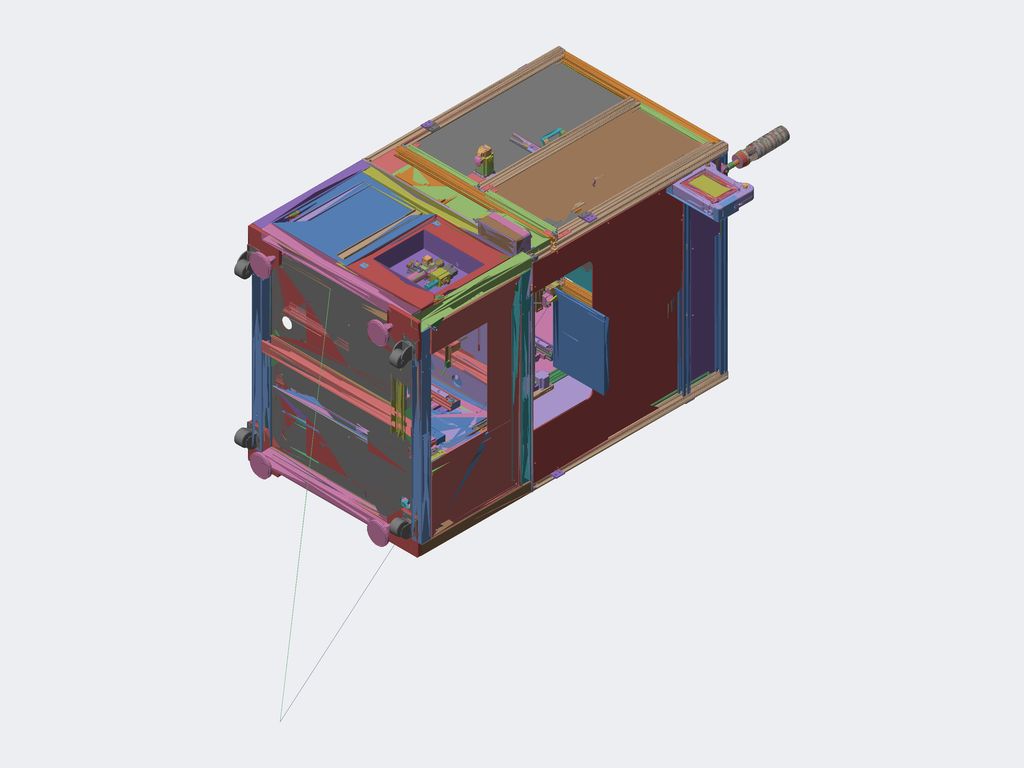Assembly | STEP file | 311 different items | 1352 placed
Parts list (item | name | quantity | parent item | size | volume):
1 | - | x3 | in standard line | 295.5 x 37 x 54 mm | 476987 mm3
2 | computer numeric keypad HW098A | x1 | - | 285 x 134.477 x 20.707 mm | 348145 mm3
3 | TOPNIKE 1205 aluminium handle, hole spacing 32mm | x1 | - | 7.369 x 16.8 x 50 mm | 4040 mm3
4 | NdFeB round magnet D12X3 with 3mm hole | x2 | - | 2.7 x 12 x 12 mm | 255.164 mm3
5 | aluminium profile door-catch magnet post | x4 | - | 14 x 14 x 37 mm | 3124 mm3
6 | monitor mounting plate | x1 | - | 92.213 x 406.803 x 260 mm | 560601 mm3
7 | magnet mounting plate | x1 | - | 20 x 12 x 35 mm | 1365 mm3
8 | smoke vent cover plate | x2 | - | 105 x 105 x 5 mm | 42706 mm3
9 | power strip mounting plate | x1 | - | 320 x 80 x 3 mm | 76368 mm3
10 | - | x4 | - | 45 x 17 x 40 mm | 3748 mm3
11 | organic panel mounting plate | x4 | - | 17 x 15 x 17 mm | 789.05 mm3
12 | - | x1 | - | 164 x 17 x 160 mm | 59024 mm3
13 | keyboard and mouse push plate | x1 | - | 14 x 138 x 548 mm | 182409 mm3
14 | 3030 L-profile sheet metal | x16 | - | 85 x 85 x 2.5 mm | 9017 mm3
15 | end cap panel MK-EC-B-4040x4.2 | x4 | in upper bracket frame assembly | 40 x 12.4 x 40 mm | 5038 mm3
16 | MK-8-4040C-L-01 profile 4040C standard 1145mm | x4 | in upper bracket frame assembly | 1145 x 40 x 40 mm | 545459 mm3
17 | - | x4 | in upper bracket frame assembly | 1120 x 40 x 40 mm | 531368 mm3
18 | MK-8-4040C-L-04 profile 4040C standard 920mm | x5 | in upper bracket frame assembly | 920 x 40 x 40 mm | 435718 mm3
19 | - | x4 | in rear door frame assembly | 1052 x 30 x 30 mm | 343124 mm3
20 | aluminium hinge 30_40 (incl. half-round hex socket bolt) | x8 | in rear door frame assembly, front door frame assembly | 66 x 54 x 16 mm | 29588 mm3
21 | - | x4 | in rear door frame assembly, front door frame assembly | 39 x 37 x 115 mm | 35258 mm3
22 | end cap panel MK-EC-B-3030x4 | x16 | in rear door frame assembly, front door frame assembly | 30 x 12.2 x 30 mm | 2778 mm3
23 | - | x8 | in rear door frame assembly, front door frame assembly | 397 x 30 x 30 mm | 129616 mm3
24 | M8x12 hex socket round-head bolt | x8 | in rear door frame assembly, front door frame assembly | 16.4 x 14 x 14 mm | 1090 mm3
25 | door panel | x2 | in rear door frame assembly | 1012 x 5 x 409 mm | 2069540 mm3
26 | MK-8-3030-L-99 profile 3030 standard 913mm | x4 | in front door frame assembly | 913 x 30 x 30 mm | 297727 mm3
27 | - | x3 | in upper bracket frame assembly | 20.75 x 39 x 18 mm | 5675 mm3
28 | - | x2 | - | 1119 x 884 x 5 mm | 3719703 mm3
29 | - | x2 | - | 1119 x 179 x 5 mm | 999682 mm3
30 | right front door acrylic cover plate | x1 | - | 870 x 409 x 5 mm | 1779111 mm3
31 | rear door acrylic cover plate | x2 | - | 1010 x 409 x 5 mm | 2065411 mm3
32 | left front door acrylic cover plate | x1 | - | 870 x 409 x 5 mm | 1779111 mm3
33 | - | x1 | - | 537 x 917 x 27.5 mm | 799133 mm3
34 | upper cover plate 2 | x1 | - | 537 x 917 x 27.5 mm | 772014 mm3
35 | spacer connection block MK-PMB-T-40 | x30 | - | 18 x 32 x 24 mm | 8600 mm3
36 | cable box hole plug φ60mm_light grey | x15 | in table top assembly | 70 x 70 x 12 mm | 8548 mm3
37 | - | x1 | - | 250 x 138 x 30 mm | 110009 mm3
38 | communication module connection plate | x1 | - | 120 x 138 x 30 mm | 59883 mm3
39 | - | x1 | - | - | -
40 | - | x1 | - | 290 x 245 x 56 mm | 381132 mm3
41 | - | x1 | - | 17.9 x 17.9 x 47.75 mm | 7538 mm3
42 | BZJ-LSX-TKJ 触摸屏MT8072iE_Default | x1 | - | - | -
43 | touch screen guide plate | x1 | - | 52 x 7.165 x 119.33 mm | 13457 mm3
44 | emergency stop button LAS1-AY-22TS-R | x1 | - | 23.995 x 49.1 x 23.995 mm | 9425 mm3
45 | - | x1 | - | 308.5 x 64.5 x 120 mm | 184454 mm3
46 | square proximity sensor GX-F12A | x4 | - | 12 x 47.7 x 8.8 mm | 2173 mm3
47 | - | x4 | - | 34.5 x 22.5 x 40 mm | 4337 mm3
48 | proximity switch mounting plate 2 | x4 | - | 40 x 32 x 18 mm | 3472 mm3
49 | display PANEL5000-IPM1502BT | x1 | - | - | -
50 | mouse | x1 | - | - | -
51 | - | x1 | - | 30.32 x 21 x 636 mm | 212983 mm3
52 | - | x2 | - | 11 x 5.5 x 5.5 mm | 119.075 mm3
53 | - | x16 | in lower bracket weldment 1000x1200 | 90 x 90 x 6 mm | 29274 mm3
54 | - | x4 | in lower bracket weldment 1000x1200 | 200 x 180 x 20 mm | 644827 mm3
55 | - | x1 | in lower bracket weldment 1000x1200 | 60 x 60 x 650 mm | 567586 mm3
56 | square steel tube 60x60x4x650 | x1 | in lower bracket weldment 1000x1200 | 60 x 60 x 650 mm | 567420 mm3
57 | square steel tube 60x60x4x880 | x2 | in lower bracket weldment 1000x1200 | 60 x 60 x 880 mm | 767950 mm3
58 | rear square steel tube 60x60x4x880 | x1 | in lower bracket weldment 1000x1200 | 60 x 60 x 880 mm | 769733 mm3
59 | - | x1 | in lower bracket weldment 1000x1200 | 60 x 60 x 880 mm | 769733 mm3
60 | - | x1 | in lower bracket weldment 1000x1200 | 60 x 60 x 1080 mm | 942814 mm3
61 | - | x1 | in lower bracket weldment 1000x1200 | 60 x 60 x 1080 mm | 943036 mm3
62 | square steel tube E60x60x4x1080 | x2 | in lower bracket weldment 1000x1200 | 60 x 60 x 1080 mm | 942050 mm3
63 | square steel tube F60x60x4x650 | x1 | in lower bracket weldment 1000x1200 | 60 x 60 x 650 mm | 567586 mm3
64 | square steel tube B60x60x4x880 | x2 | in lower bracket weldment 1000x1200 | 60 x 60 x 880 mm | 770145 mm3
65 | - | x1 | in lower bracket weldment 1000x1200 | 60 x 60 x 650 mm | 580718 mm3
66 | table plate | x1 | in lower bracket weldment 1000x1200 | 1000 x 1200 x 10 mm | 11534031 mm3
67 | - | x1 | in lower bracket weldment 1000x1200 | 45 x 5 x 105 mm | 23005 mm3
68 | spacer plate 4 | x1 | in lower bracket weldment 1000x1200 | 56 x 5 x 105 mm | 28583 mm3
69 | spacer plate 4 | x1 | in lower bracket weldment 1000x1200 | 56 x 5 x 105 mm | 28583 mm3
70 | - | x1 | in lower bracket weldment 1000x1200 | 45 x 5 x 105 mm | 23005 mm3
71 | - | x1 | in lower bracket weldment 1000x1200 | 105 x 5 x 105 mm | 53833 mm3
72 | - | x1 | in lower bracket weldment 1000x1200 | 105 x 5 x 105 mm | 53833 mm3
73 | - | x4 | in lower frame assembly 1000x1200 | 120 x 147 x 120 mm | 298172 mm3
74 | - | x4 | in lower frame assembly 1000x1200 | 112 x 105 x 88 mm | 158459 mm3
75 | - | x2 | in lower frame door assembly | 18 x 17 x 130 mm | 7934 mm3
76 | cylinder lock MS813-Shengjiu | x4 | in lower frame door assembly | 58.793 x 35 x 31.6 mm | 16415 mm3
77 | - | x2 | in lower frame door assembly | 15 x 20 x 350 mm | 20205 mm3
78 | - | x1 | - | 446.8 x 526 x 18.2 mm | 391845 mm3
79 | hinge CL237Z3H001-01 | x8 | in hinge CL237Z3H001 | 17.5 x 48 x 18 mm | 5234 mm3
80 | - | x8 | in hinge CL237Z3H001 | 19 x 25 x 8.5 mm | 1495 mm3
81 | - | x1 | - | 436 x 526 x 17 mm | 186343 mm3
82 | air source assembly mounting plate | x1 | - | 365 x 304.8 x 102 mm | 354021 mm3
83 | hand slide valve HSV08 | x1 | - | - | -
84 | - | x2 | - | 39.583 x 28.8 x 17.7 mm | 7284 mm3
85 | T-bracket GA300T-P1 | x1 | - | 60.5 x 88 x 12.5 mm | 30830 mm3
86 | soft-start valve GV30008JF1B | x1 | - | 57.4 x 130.9 x 74 mm | 252989 mm3
87 | plastic foam silencer PAL-03 | x1 | - | 26 x 68 x 26.213 mm | 26024 mm3
88 | pressure regulating filter GFR300-08-N | x1 | - | - | -
89 | digital pressure switch DP-102 | x1 | - | 30 x 30 x 44.8 mm | 24470 mm3
90 | countersunk screw spacer block | x16 | in lower frame bottom cover plate assembly, lower frame left cover plate assembly | 15 x 17 x 15 mm | 1639 mm3
91 | lower frame bottom cover plate | x2 | in lower frame bottom cover plate assembly | - | -
92 | lower frame left cover plate | x1 | in lower frame left cover plate assembly | 527 x 1077 x 15 mm | 446588 mm3
93 | - | x1 | - | 527 x 1077 x 15 mm | 446588 mm3
94 | table plate | x1 | in table top assembly | 1000 x 1200 x 10 mm | 11534031 mm3
95 | - | x10 | in assembled motion assembly | 15 x 18.7 x 22 mm | 803.602 mm3
96 | - | x5 | in assembled motion assembly | 15 x 19 x 15 mm | 469.105 mm3
97 | - | x5 | in assembled motion assembly | 35 x 35 x 10 mm | 7611 mm3
98 | Y-axis cable chain support plate | x1 | in assembled motion assembly | 327 x 8 x 80 mm | 201857 mm3
99 | Y-axis cable chain mounting plate (hole pitch 87) | x1 | in assembled motion assembly | 52.3 x 96 x 100 mm | 42065 mm3
100 | X-axis connection reinforcing block | x1 | in assembled motion assembly | 300 x 86 x 32 mm | 534000 mm3
101 | X-axis mounting plate | x1 | in assembled motion assembly | 533 x 86 x 35 mm | 1297130 mm3
102 | energy chain clamp plate | x1 | in assembled motion assembly | 137 x 78 x 48.5 mm | 25843 mm3
103 | - | x1 | in assembled motion assembly | 37.5 x 25 x 220 mm | 19433 mm3
104 | - | x1 | in assembled motion assembly | 139.01 x 140 x 74.02 mm | 52784 mm3
105 | - | x1 | in assembled motion assembly | 66 x 220 x 12 mm | 169355 mm3
106 | - | x1 | in assembled motion assembly | 95 x 4 x 110 mm | 40723 mm3
107 | energy chain mounting plate | x1 | in assembled motion assembly | 78 x 5 x 40 mm | 14101 mm3
108 | - | x1 | in assembled motion assembly | 300 x 100 x 22 mm | 536416 mm3
109 | Y-axis module mounting plate 590 | x1 | in assembled motion assembly | 86 x 745 x 36 mm | 2257304 mm3
110 | - | x2 | in assembled motion assembly | 61 x 63 x 10 mm | 20131 mm3
111 | KR3310A-0100-0-10A0 rail | x1 | - | 270 x 48.2 x 62 mm | 372250 mm3
112 | KR3310A-10A0 carriage | x1 | - | 54 x 15 x 86 mm | 46318 mm3
113 | double-diaphragm coupling LC-A-025DA-06B-14B-T001 | x1 | in assembled motion assembly | 32.8 x 27 x 27 mm | 11316 mm3
114 | - | x9 | in assembled motion assembly, bottom return line assembly | 22.7 x 14.9 x 13.4 mm | 1660 mm3
115 | module KR050 photoelectric mounting profile 150 | x1 | in assembled motion assembly | 8 x 5 x 150 mm | 2740 mm3
116 | - | x2 | in assembled motion assembly | 48 x 39 x 39 mm | 40714 mm3
117 | - | x1 | - | 740.5 x 67.1 x 90.55 mm | 1776766 mm3
118 | - | x2 | - | 81 x 22 x 112 mm | 111956 mm3
119 | - | x2 | - | 13.9 x 27.5 x 16 mm | 2147 mm3
120 | - | x2 | - | 86 x 63.5 x 8 mm | 28261 mm3
121 | KK86 stepper coupling flange | x2 | - | 86 x 63.5 x 8 mm | 31412 mm3
122 | I/O terminal box 23N8S1 | x1 | in assembled motion assembly | - | -
123 | - | x1 | - | 440.5 x 67.1 x 95.1 mm | 1162435 mm3
124 | - | x2 | in assembled motion assembly | 375 x 150 x 77.5 mm | 1474112 mm3
125 | - | x1 | in assembled motion assembly | 94 x 145 x 792.5 mm | 1305245 mm3
126 | - | x2 | in assembled motion assembly | 63.062 x 154.188 x 80 mm | 326216 mm3
127 | - | x4 | in assembled motion assembly | 15 x 15 x 3.2 mm | 292.86 mm3
128 | - | x1 | in assembled motion assembly | 63.062 x 188.688 x 80 mm | 431476 mm3
129 | Z-axis assembly mounting plate | x1 | in assembled motion assembly | 180 x 150 x 12 mm | 304023 mm3
130 | vacuum generator mounting plate 2 | x1 | in assembled motion assembly | 50 x 3 x 110 mm | 12230 mm3
131 | cable chain hanger plate 2 | x1 | in assembled motion assembly | 3 x 95 x 164 mm | 41712 mm3
132 | Siemens 400W motor mounting plate | x1 | in assembled motion assembly | 64 x 12 x 64 mm | 33213 mm3
133 | - | x1 | in assembled motion assembly | 80 x 187 x 15 mm | 46500 mm3
134 | - | x1 | in assembled motion assembly | - | -
135 | junction box mounting plate | x1 | in table top assembly | 130 x 136.5 x 127.074 mm | 85918 mm3
136 | IO-LINK slave M12 Hub 16xDI-DO NPN | x2 | in table top assembly | - | -
137 | - | x8 | - | 141.7 x 32.5 x 16 mm | 47379 mm3
138 | - | x4 | - | 17 x 46.3 x 15 mm | 6244 mm3
139 | - | x1 | - | 22.8 x 57.5 x 146 mm | 85064 mm3
140 | - | x1 | - | 86.5 x 113.075 x 190 mm | 98833 mm3
141 | - | x1 | - | 35.315 x 34 x 18 mm | 5648 mm3
142 | - | x16 | - | 11.547 x 10 x 20 mm | 1033 mm3
143 | 982 blanking plug (1-8 plug) | x1 | - | 10 x 6.95 x 10 mm | 421.396 mm3
144 | small support plate_sandblasted anodised | x2 | in forward-flow width adjuster assembly_chain | 20 x 80 x 80 mm | 64176 mm3
145 | - | x2 | in forward-flow width adjuster assembly_chain | 20 x 97 x 80 mm | 92738 mm3
146 | moving support plate_sandblasted anodised | x2 | in forward-flow width adjuster assembly_chain | 20 x 95 x 90 mm | 73168 mm3
147 | - | x2 | in forward-flow width adjuster assembly_chain | 20 x 20 x 505 mm | 158440 mm3
148 | - | x3 | in forward-flow width adjuster assembly_chain | 40 x 28 x 2 mm | 1349 mm3
149 | - | x3 | in forward-flow width adjuster assembly_chain | 40 x 30 x 2 mm | 1364 mm3
150 | - | x3 | in forward-flow width adjuster assembly_chain | 26 x 26 x 8 mm | 2544 mm3
151 | guided double-liner flanged linear bearing LML21-d20 | x4 | in forward-flow width adjuster assembly_chain | 80 x 54 x 38 mm | 45928 mm3
152 | - | x2 | in forward-flow width adjuster assembly_chain | 3 x 3 x 14 mm | 119.894 mm3
153 | rail-02 nut SFU01604-4 | x3 | in ball screw SFUR1604-565 | 40 x 40 x 48 mm | 25660 mm3
154 | - | x2 | - | 16 x 16 x 545 mm | 99221 mm3
155 | - | x3 | in forward-flow width adjuster assembly_chain | 28 x 28 x 8 mm | 3776 mm3
156 | - | x3 | in forward-flow width adjuster assembly_chain | 22 x 22 x 8 mm | 1773 mm3
157 | - | x2 | in forward-flow width adjuster assembly_chain | 37 x 19 x 37 mm | 15386 mm3
158 | - | x2 | in side guide-wheel chain conveyor_front | 110 x 21 x 64 mm | 49771 mm3
159 | - | x8 | in BZJ-LSX-TKJ 链条惰轮Component-30 | 31 x 9 x 31 mm | 3611 mm3
160 | - | x16 | in BZJ-LSX-TKJ 链条惰轮Component-30, BZJ-LSX-TKJ 链条惰轮Component-25 | 6 x 17 x 17 mm | 776.566 mm3
161 | - | x16 | in BZJ-LSX-TKJ 链条惰轮Component-30, BZJ-LSX-TKJ 链条惰轮Component-25 | 18.3 x 17.603 x 1 mm | 85.781 mm3
162 | sprocket spacer | x4 | in side guide-wheel chain conveyor_front | 15 x 15 x 6.2 mm | 541.108 mm3
163 | - | x1 | in side guide-wheel chain conveyor_front | 35 x 55 x 1000 mm | 772686 mm3
164 | line front chain guide channel L800 | x1 | in side guide-wheel chain conveyor_front | 35 x 55 x 1000 mm | 772686 mm3
165 | - | x8 | in BZJ-LSX-TKJ 链条惰轮Component-25 | 25 x 8.5 x 25 mm | 1521 mm3
166 | - | x4 | in side guide-wheel chain conveyor_front, 06B side guide-wheel chain conveyor | 34.8 x 1 x 54.8 mm | 1804 mm3
167 | - | x4 | in side guide-wheel chain conveyor_front, 06B side guide-wheel chain conveyor | 34.8 x 1 x 54.8 mm | 1804 mm3
168 | - | x8 | in side guide-wheel chain conveyor_front, 06B side guide-wheel chain conveyor | 15 x 15 x 3.5 mm | 281.21 mm3
169 | driven guide-wheel connector | x8 | in side guide-wheel chain conveyor_front, 06B side guide-wheel chain conveyor | 36 x 5 x 10.6 mm | 1667 mm3
170 | 06B side guide-wheel chain support block | x4 | in side guide-wheel chain conveyor_front, 06B side guide-wheel chain conveyor | 9 x 900 x 20.4 mm | 141982 mm3
171 | plain key type A GB_T 1096-key 3x3x12 | x4 | in side guide-wheel chain conveyor_front, 06B side guide-wheel chain conveyor | 12 x 3 x 3 mm | 101.479 mm3
172 | drive sprocket 06B-10 teeth_bore φ10 | x4 | in side guide-wheel chain conveyor_front, 06B side guide-wheel chain conveyor | 34 x 32.715 x 12 mm | 4151 mm3
173 | - | x5 | in side guide-wheel chain conveyor_front, 06B side guide-wheel chain conveyor, bottom return line assembly | 60 x 96 x 60 mm | 237550 mm3
174 | 06B side guide-wheel chain | x448 | in side guide-wheel chain conveyor_front, 06B side guide-wheel chain conveyor | 18.325 x 9 x 17.4 mm | 854.513 mm3
175 | photoelectric mounting plate 2 | x2 | in side guide-wheel chain conveyor_front | 33 x 38 x 75 mm | 6071 mm3
176 | - | x4 | in side guide-wheel chain conveyor_front | 30 x 58.715 x 105.315 mm | 11448 mm3
177 | lift mounting plate 2 | x2 | in lift assembly | 180 x 20 x 52 mm | 120822 mm3
178 | lift adapter plate 2 | x2 | in lift assembly | 210 x 10 x 52 mm | 101060 mm3
179 | - | x4 | in lift assembly | 8.5 x 30 x 8.5 mm | 658.629 mm3
180 | - | x4 | in rail MGN9C1R-45-Z1CM | 9 x 6.5 x 45 mm | 2232 mm3
181 | - | x6 | in rail MGN9C1R-45-Z1CM, rail MGN9C1R-37-Z1CM | 20 x 8 x 29 mm | 3311 mm3
182 | - | x2 | in lift assembly | 270 x 98 x 6 mm | 118371 mm3
183 | polyurethane anti-collision post | x4 | in lift assembly | 12 x 14.5 x 12 mm | 1232 mm3
184 | linear rail mounting plate | x1 | - | 150 x 35 x 38 mm | 166586 mm3
185 | rail-01 MGN9C1R-37-Z1CM_PERSON_A hot-press welding configuration | x2 | in rail MGN9C1R-37-Z1CM | 9 x 6.5 x 37 mm | 1790 mm3
186 | - | x1 | - | 57 x 24.2 x 16.7 mm | 11440 mm3
187 | - | x2 | - | 9.373 x 25.4 x 22 mm | 1869 mm3
188 | side push plate | x1 | - | 270 x 4 x 75 mm | 59912 mm3
189 | side push connection plate | x1 | - | 40 x 18 x 9 mm | 1135 mm3
190 | - | x1 | - | 9 x 9 x 5.8 mm | 258.691 mm3
191 | - | x2 | in side guide-wheel chain conveyor_front | 30 x 13 x 30 mm | 5307 mm3
192 | photoelectric shutter | x2 | in side guide-wheel chain conveyor_front, bottom return line assembly | 8 x 40.1 x 11.1 mm | 333.086 mm3
193 | - | x2 | in side guide-wheel chain conveyor_front, 06B side guide-wheel chain conveyor | 15 x 1 x 7 mm | 49.292 mm3
194 | upper limit plate 1 | x1 | in side guide-wheel chain conveyor_front | 326 x 11 x 40 mm | 109712 mm3
195 | upper limit plate 2 | x1 | in side guide-wheel chain conveyor_front | 326 x 11 x 40 mm | 72637 mm3
196 | - | x3 | - | - | -
197 | stop bar | x3 | - | 14 x 5 x 94 mm | 6342 mm3
198 | bar cover plate | x3 | - | 70 x 4 x 38 mm | 9112 mm3
199 | cylinder mounting plate | x3 | - | 38 x 32 x 38 mm | 17881 mm3
200 | M3x8 socket head cap screw | x21 | - | 5.5 x 11 x 5.5 mm | 105.547 mm3
201 | miniature tube fitting M-3ALU-4 | x6 | - | 5 x 9.5 x 10.687 mm | 200.167 mm3
202 | - | x3 | - | 34 x 22 x 13.5 mm | 6493 mm3
203 | - | x3 | - | 4 x 4 x 4.1 mm | 14.297 mm3
204 | bar mounting plate | x3 | - | 19 x 37 x 4 mm | 1217 mm3
205 | - | x2 | in side guide-wheel chain conveyor_front | 33 x 50 x 27 mm | 3903 mm3
206 | - | x3 | in side guide-wheel chain conveyor_front, bottom return line assembly | 27.685 x 9 x 17.043 mm | 1685 mm3
207 | cable chain J15BF.1.20N28 1 | x1 | in table top assembly | 28.5 x 74.5 x 367.25 mm | 251972 mm3
208 | cable chain mounting sheet metal 1 | x1 | in table top assembly | 30 x 50 x 30 mm | 4308 mm3
209 | - | x2 | in table top assembly | 57 x 79 x 57 mm | 128182 mm3
210 | - | x2 | in table top assembly | 95 x 155 x 20 mm | 30386 mm3
211 | motor mounting sheet metal 2 | x1 | in table top assembly | 58 x 15 x 55 mm | 5412 mm3
212 | cover plate 1 | x2 | in table top assembly | 65 x 153 x 1 mm | 9370 mm3
213 | - | x2 | in table top assembly | 122.93 x 36.98 x 8 mm | 5373 mm3
214 | timing pulley 16-3M-Φ10-18 | x2 | in table top assembly | 17.5 x 18 x 17.5 mm | 1873 mm3
215 | - | x4 | in table top assembly | 85 x 75 x 75 mm | 250465 mm3
216 | mounting assembly column ZCD06-D50-L350 | x2 | in table top assembly | 50 x 50 x 350 mm | 350484 mm3
217 | - | x1 | in table top assembly | 105 x 5 x 105 mm | 53833 mm3
218 | - | x1 | in table top assembly | 105 x 5 x 105 mm | 53833 mm3
219 | - | x1 | in table top assembly | 45 x 5 x 105 mm | 23005 mm3
220 | - | x1 | in table top assembly | 45 x 5 x 105 mm | 23005 mm3
221 | spacer plate 4 | x1 | in table top assembly | 56 x 5 x 105 mm | 28583 mm3
222 | spacer plate 4 | x1 | in table top assembly | 56 x 5 x 105 mm | 28583 mm3
223 | straight dowel pin 6x12 (g tolerance) | x20 | in table top assembly | 6 x 6 x 12 mm | 338.555 mm3
224 | lift mounting plate | x1 | - | 200 x 11 x 435 mm | 935610 mm3
225 | - | x4 | - | 20 x 20 x 145 mm | 45098 mm3
226 | bearing LMF20LUU | x4 | - | 54 x 80 x 54 mm | 49091 mm3
227 | - | x1 | - | 9 x 85 x 65 mm | 34372 mm3
228 | - | x2 | - | 13 x 30.6 x 26.1 mm | 3953 mm3
229 | slim cylinder SDA32x15S | x1 | - | 56.5 x 44 x 50 mm | 73999 mm3
230 | pivot pin bolt DBS6-6-8 | x1 | - | 18 x 16 x 16 mm | 1445 mm3
231 | front return support plate | x1 | - | 835 x 60 x 15 mm | 710193 mm3
232 | rear return support plate | x1 | - | 835 x 60 x 15 mm | 730825 mm3
233 | - | x2 | - | 20 x 20 x 530 mm | 164323 mm3
234 | - | x1 | - | 90 x 60 x 20 mm | 50932 mm3
235 | front rail support plate | x2 | - | 74.6 x 15 x 47 mm | 42579 mm3
236 | linear bearing mounting plate | x2 | - | 90 x 60 x 20 mm | 49506 mm3
237 | - | x1 | in ball screw SFUR1604-565 | 16 x 16 x 565 mm | 102973 mm3
238 | photoelectric mounting plate | x1 | in bottom return line assembly | 36 x 15 x 50 mm | 3316 mm3
239 | - | x2 | in 06B side guide-wheel chain conveyor | 35 x 55 x 1000 mm | 771122 mm3
240 | - | x2 | in 06B side guide-wheel chain conveyor | 139 x 65 x 48 mm | 36917 mm3
241 | - | x4 | in 06B side guide-wheel chain conveyor | 15 x 15 x 13.2 mm | 775.094 mm3
242 | hexagon socket head cap screws gb_PreviewCfg | x4 | in 06B side guide-wheel chain conveyor | 7.6 x 3 x 3 mm | 21.652 mm3
243 | - | x1 | in 06B side guide-wheel chain conveyor | 43 x 13 x 13 mm | 2644 mm3
244 | - | x2 | in 06B side guide-wheel chain conveyor | 11.2 x 58.715 x 100.215 mm | 7246 mm3
245 | - | x2 | in 06B side guide-wheel chain conveyor | 18.5 x 102 x 16 mm | 4317 mm3
246 | - | x2 | in bottom return line assembly | 30 x 30 x 5 mm | 2041 mm3
247 | - | x1 | in bottom return line assembly | 90 x 60 x 54 mm | 30144 mm3
248 | - | x1 | in bottom return line assembly | 550 x 30 x 73.5 mm | 112714 mm3
249 | cable chain mounting plate | x1 | in bottom return line assembly | 30 x 70 x 50 mm | 6708 mm3
250 | double-diaphragm coupling LC-A-030DA-10B-10B | x1 | in bottom return line assembly | 34 x 34 x 37.8 mm | 23948 mm3
251 | cable chain J15BF.1.20N28 | x1 | in bottom return line assembly | 28.5 x 74.5 x 367.25 mm | 251972 mm3
252 | - | x4 | in bottom return line assembly | - | -
253 | - | x1 | in bottom return line assembly | 29.939 x 86.939 x 25.75 mm | 39070 mm3
254 | lower return mounting plate | x4 | in bottom return line assembly | 53 x 50 x 109.5 mm | 39119 mm3
255 | component mounting plate | x1 | - | 817 x 435 x 20 mm | 536830 mm3
256 | - | x1 | - | - | -
257 | power filter DL-10T1 | x1 | - | 89.5 x 36.5 x 51.5 mm | 121807 mm3
258 | miniature circuit breaker IC65N-2P-C16A | x1 | - | 35.4 x 93.9 x 74.3 mm | 159125 mm3
259 | - | x1 | - | 17.5 x 90.6 x 73.848 mm | 76092 mm3
260 | - | x1 | - | 76.2 x 105.618 x 73.908 mm | 172435 mm3
261 | Schneider AC contactor (24V coil) LC1D09BDC | x1 | - | - | -
262 | - | x1 | - | 54 x 38 x 11.5 mm | 8666 mm3
263 | - | x1 | - | 85 x 115 x 44.75 mm | 205156 mm3
264 | fuse terminal PT4-HESILED24(5x20)-3211903 | x2 | - | 6.15 x 55.9 x 63.38 mm | 12999 mm3
265 | feed-through terminal PT 1.5-S-QUATTRO | x40 | - | 3.5 x 63.2 x 30.5 mm | 4808 mm3
266 | - | x6 | - | 6.2 x 88.87 x 77.9 mm | 26675 mm3
267 | feed-through terminal PT2,5-QUATTRO-3209578 | x12 | - | 5.15 x 72.2 x 35.25 mm | 9561 mm3
268 | servo drive SV660PS1R6I | x2 | - | 40 x 213 x 175.4 mm | 974697 mm3
269 | - | x1 | - | 40 x 212 x 175.4 mm | 959953 mm3
270 | - | x1 | - | - | -
271 | - | x1 | - | - | -
272 | IO expansion module HCB2-1616-DTD01 | x1 | - | 120.4 x 65 x 97 mm | 571916 mm3
273 | rail switch-mode power supply NDR-240-24 | x1 | - | 124.256 x 63 x 128.712 mm | 109932 mm3
274 | PILZ safety relay PNOZX2 | x2 | - | 87.8 x 22.5 x 120.6 mm | 199420 mm3
275 | 5-port DIN-rail switch EDS-205 | x1 | - | 98.5 x 110.5 x 24.9 mm | 215104 mm3
276 | - | x3 | - | 5.5 x 35 x 230 mm | 4835 mm3
277 | 35 wire duct_552 | x1 | - | 50.625 x 35 x 552 mm | 74720 mm3
278 | 35 wire duct_425 | x2 | - | 50.625 x 35 x 425 mm | 57556 mm3
279 | 35 wire duct | x2 | - | 50.625 x 35 x 366 mm | 49541 mm3
280 | 35 wire duct_314 | x2 | - | 50.625 x 35 x 314 mm | 42522 mm3
281 | - | x1 | - | 489 x 202 x 10 mm | 164472 mm3
282 | - | x1 | - | 50.625 x 35 x 384 mm | 51986 mm3
283 | 35 wire duct_410 | x3 | - | 50.625 x 35 x 410 mm | 55518 mm3
284 | 35 wire duct_200 | x2 | - | 50.625 x 35 x 200 mm | 27080 mm3
285 | DIN rail L60 | x1 | - | 5.5 x 35 x 80 mm | 1674 mm3
286 | - | x2 | - | 30 x 30 x 1 mm | 412.566 mm3
287 | class B ventilation filter unit ZL-803 (7032 adhesive) | x2 | - | 150 x 150 x 28 mm | 421271 mm3
288 | cabinet brush KEL-BES-S24 | x14 | - | 148 x 10 x 58 mm | 60298 mm3
289 | - | x2 | - | 120 x 120 x 38 mm | 111801 mm3
290 | - | x1 | - | - | -
291 | - | x4 | in electrical cabinet right door weldment, electrical cabinet left door weldment | 390 x 21 x 6 mm | 9834 mm3
292 | right door panel 2 | x1 | in electrical cabinet right door weldment | 435.5 x 525.8 x 17 mm | 303156 mm3
293 | - | x4 | in electrical cabinet right door weldment, electrical cabinet left door weldment | 350 x 21 x 6 mm | 8835 mm3
294 | left sheet-metal door panel | x1 | in electrical cabinet left door weldment | 444.3 x 525.8 x 20.2 mm | 297154 mm3
295 | power knob mounting sheet metal | x1 | in electrical cabinet left door weldment | 74 x 122 x 41 mm | 24069 mm3
296 | LED lamp for distribution cabinet QELTS-500-220 | x1 | in electrical cabinet assembly | 37 x 33.2 x 578 mm | 564522 mm3
297 | indicator light AD17-22-AC220VW white | x1 | in electrical cabinet assembly | 29 x 29.009 x 63.018 mm | 10026 mm3
298 | - | x1 | in electrical cabinet assembly | - | -
299 | SMEMA connector | x2 | in electrical cabinet assembly | 36 x 36 x 78.52 mm | 45655 mm3
300 | interface connection plate | x1 | in electrical cabinet assembly | 350 x 81.5 x 31.5 mm | 67618 mm3
301 | four-hole button box TYX4 | x1 | in 4-hole button box assembly | 220 x 85 x 75 mm | 244482 mm3
302 | - | x1 | in 4-hole button box assembly | 40 x 40 x 48 mm | 24355 mm3
303 | push-button head LA42PD-G | x1 | in 4-hole button box assembly | 30 x 30 x 33 mm | 18043 mm3
304 | - | x1 | in 4-hole button box assembly | 30 x 30 x 76 mm | 18961 mm3
305 | - | x1 | in 4-hole button box assembly | 30 x 30 x 33 mm | 18043 mm3
306 | connection bracket LA42-PT-ZJ | x4 | in 4-hole button box assembly | 41 x 30 x 22 mm | 6377 mm3
307 | switch contact LA42-01-NC | x4 | in 4-hole button box assembly | 32 x 10 x 42 mm | 10410 mm3
308 | - | x4 | in 4-hole button box assembly | 32 x 10 x 42 mm | 10410 mm3
309 | push-button box mounting plate | x1 | in 4-hole button box assembly | 220 x 108.5 x 78 mm | 90266 mm3
310 | Schneider emergency stop button guard ZB2BZ1605C | x1 | in 4-hole button box assembly | 50 x 30 x 50 mm | 7549 mm3
311 | PN_0004 jig | x1 | in standard line | 400 x 30 x 300 mm | 3171570 mm3
Placements (level | parent | child | x y z in mm | rotation matrix by rows), first 252 of 1427 lines:
1 | standard line | subassembly 2 | -1539.317 2392.592 -683.387 | 1 0 0 0 1 0 0 0 1
2 | subassembly 2 | subassembly 3 | 1365.143 95.729 1587.458 | 0 -1 0 0 0 -1 1 0 -0
2 | subassembly 2 | computer numeric keypad HW098A | 578.143 -765.655 2158.584 | 1 0 0 0 1 -0.007187 0 0.007187 1
2 | subassembly 2 | TOPNIKE 1205 aluminium handle, hole spacing 32mm | 843.143 -645.88 2190.246 | 0 0 -1 -1 -0.007187 0 -0.007187 1 0
2 | subassembly 2 | NdFeB round magnet D12X3 with 3mm hole | 898.143 -636.771 2166.999 | 0 -0.8051 -0.5931 0 0.5931 -0.8051 1 0 -0
2 | subassembly 2 | NdFeB round magnet D12X3 with 3mm hole | 918.143 -636.771 2166.999 | 0 -0.8051 -0.5931 0 0.5931 -0.8051 1 0 -0
2 | subassembly 2 | aluminium profile door-catch magnet post | 878.143 320.229 1025.699 | -1 0 0 0 1 0 0 0 -1
2 | subassembly 2 | aluminium profile door-catch magnet post | 938.143 320.229 2135.699 | 1 0 0 0 1 0 0 0 1
2 | subassembly 2 | aluminium profile door-catch magnet post | 878.143 320.229 2135.699 | 1 0 0 0 1 0 0 0 1
2 | subassembly 2 | monitor mounting plate | 553.143 371.229 2135.699 | 0 0 1 0 1 0 -1 0 0
2 | subassembly 2 | magnet mounting plate | 908.143 -629.771 2166.999 | 0 0 -1 0 1 0 1 0 -0
2 | subassembly 2 | smoke vent cover plate | 568.143 380.229 1164.199 | 1 0 0 0 0 -1 0 1 -0
2 | subassembly 2 | power strip mounting plate | 1368.143 105.229 1583.458 | 0 0 1 0 1 0 -1 0 -0
2 | subassembly 2 | subassembly 4 | 878.143 334.229 1022.699 | 0 0 -1 -1 0 0 0 1 -0
2 | subassembly 2 | subassembly 4 | 938.143 334.229 2138.699 | 0 0 1 -1 0 0 0 -1 0
2 | subassembly 2 | subassembly 4 | 878.143 334.229 2138.699 | 0 0 1 -1 0 0 0 -1 0
2 | subassembly 2 | organic panel mounting plate | 430.143 -767.771 1121.199 | -1 0 0 0 0 -1 0 -1 -0
2 | subassembly 2 | organic panel mounting plate | 430.143 -767.771 2020.199 | -1 0 0 0 0 -1 0 -1 -0
2 | subassembly 2 | organic panel mounting plate | 1386.143 -767.771 2020.199 | 1 0 0 0 0 -1 0 1 -0
2 | subassembly 2 | organic panel mounting plate | 1386.143 -767.771 1121.199 | 1 0 0 0 0 -1 0 1 -0
2 | subassembly 2 | subassembly 5 | 1021.143 -673.771 2138.699 | -1 0 0 0 0 -1 0 -1 -0
2 | subassembly 2 | keyboard and mouse push plate | 843.143 -726.564 2180.866 | 0 0 -1 -0.007187 1 0 1 0.007187 0
2 | subassembly 2 | 3030 L-profile sheet metal | 912.143 331.229 2148.199 | 0 1 0 -1 0 0 0 0 1
2 | subassembly 2 | 3030 L-profile sheet metal | 904.143 331.229 2148.199 | -1 0 0 0 -1 0 0 0 1
2 | subassembly 2 | 3030 L-profile sheet metal | 1365.143 331.229 2148.199 | -1 0 0 0 -1 0 0 0 1
2 | subassembly 2 | 3030 L-profile sheet metal | 451.143 331.229 2150.699 | 1 0 0 0 -1 0 0 0 -1
2 | subassembly 2 | 3030 L-profile sheet metal | 451.143 330.729 1010.831 | 1 0 0 0 -1 0 0 0 -1
2 | subassembly 2 | 3030 L-profile sheet metal | 904.143 330.729 1008.331 | -1 0 0 0 -1 0 0 0 1
2 | subassembly 2 | 3030 L-profile sheet metal | 904.143 -585.771 2150.699 | -1 0 0 0 1 0 0 0 -1
2 | subassembly 2 | 3030 L-profile sheet metal | 912.143 -585.771 2148.199 | 1 0 0 0 1 0 0 0 1
2 | subassembly 2 | 3030 L-profile sheet metal | 451.143 -585.771 2148.199 | 1 0 0 0 1 0 0 0 1
2 | subassembly 2 | 3030 L-profile sheet metal | 1365.143 -585.771 2150.699 | -1 0 0 0 1 0 0 0 -1
2 | subassembly 2 | 3030 L-profile sheet metal | 451.143 -725.271 1008.331 | 1 0 0 0 1 0 0 0 1
2 | subassembly 2 | 3030 L-profile sheet metal | 904.143 -725.271 1010.831 | -1 0 0 0 1 0 0 0 -1
2 | subassembly 2 | subassembly 6 | 380.103 -837.624 626.003 | 1 0 0 0 1 0 0 0 1
3 | subassembly 6 | upper bracket frame assembly | -291.856 1200.854 1504.696 | 1 0 0 0 1 0 0 0 1
4 | upper bracket frame assembly | end cap panel MK-EC-B-4040x4.2 | 1299.896 16.2 30.0 | -1 0 0 0 -1 0 0 0 1
4 | upper bracket frame assembly | end cap panel MK-EC-B-4040x4.2 | 1299.896 16.2 -1130.0 | -1 0 0 0 -1 0 0 0 1
4 | upper bracket frame assembly | end cap panel MK-EC-B-4040x4.2 | 339.896 16.2 -1130.0 | -1 0 0 0 -1 0 0 0 1
4 | upper bracket frame assembly | end cap panel MK-EC-B-4040x4.2 | 339.896 16.2 30.0 | -1 0 0 0 -1 0 0 0 1
4 | upper bracket frame assembly | MK-8-4040C-L-01 profile 4040C standard 1145mm | 1299.896 -1133.0 30.0 | 0 0 -1 1 0 0 0 -1 0
4 | upper bracket frame assembly | MK-8-4040C-L-01 profile 4040C standard 1145mm | 1299.896 -1133.0 -1130.0 | 0 0 1 1 0 0 0 1 -0
4 | upper bracket frame assembly | MK-8-4040C-L-01 profile 4040C standard 1145mm | 339.896 -1133.0 30.0 | 0 0 -1 1 0 0 0 -1 -0
4 | upper bracket frame assembly | MK-8-4040C-L-01 profile 4040C standard 1145mm | 339.896 -1133.0 -1130.0 | 0 0 -1 1 0 0 0 -1 -0
4 | upper bracket frame assembly | subassembly 7 | 1299.896 -228.0 10.0 | 0 1 0 0 0 -1 -1 0 -0
4 | upper bracket frame assembly | subassembly 7 | 1299.896 -8.0 10.0 | 0 -1 0 0 0 1 -1 0 0
4 | upper bracket frame assembly | subassembly 7 | 339.896 -8.0 10.0 | 0 1 0 0 0 -1 -1 0 -0
4 | upper bracket frame assembly | subassembly 7 | 339.896 -228.0 10.0 | 0 1 0 0 0 -1 -1 0 -0
4 | upper bracket frame assembly | MK-8-4040C-L-04 profile 4040C standard 920mm | 359.896 -973.0 30.0 | 1 0 0 0 0 -1 0 1 -0
4 | upper bracket frame assembly | MK-8-4040C-L-04 profile 4040C standard 920mm | 359.896 -8.0 30.0 | 1 0 0 0 0 -1 0 1 -0
4 | upper bracket frame assembly | MK-8-4040C-L-04 profile 4040C standard 920mm | 359.896 -8.0 -1130.0 | 1 0 0 0 0 -1 0 1 -0
4 | upper bracket frame assembly | MK-8-4040C-L-04 profile 4040C standard 920mm | 359.896 -8.0 -550.0 | 1 0 0 0 -1 0 0 0 -1
4 | upper bracket frame assembly | rear door frame assembly | 367.017 -940.671 -1109.427 | 1 0 0 0 -1 0 0 0 -1
5 | rear door frame assembly | subassembly 8 | 8.879 145.829 27.942 | 0 0 1 -1 0 0 0 -1 0
5 | rear door frame assembly | subassembly 8 | 435.879 145.829 27.942 | 0 0 1 -1 0 0 0 -1 0
5 | rear door frame assembly | aluminium hinge 30_40 (incl. half-round hex socket bolt) | -5.271 -24.171 42.942 | 1 0 0 0 1 0 0 0 1
5 | rear door frame assembly | aluminium hinge 30_40 (incl. half-round hex socket bolt) | -5.271 -786.171 42.942 | 1 0 0 0 1 0 0 0 1
5 | rear door frame assembly | subassembly 9 | 445.879 -380.171 42.942 | -1 0 0 0 0 -1 0 -1 -0
5 | rear door frame assembly | end cap panel MK-EC-B-3030x4 | 8.879 149.829 27.942 | 0 0 -1 0 -1 0 -1 0 -0
5 | rear door frame assembly | end cap panel MK-EC-B-3030x4 | 435.879 149.829 27.942 | 0 0 -1 0 -1 0 -1 0 -0
5 | rear door frame assembly | end cap panel MK-EC-B-3030x4 | 435.879 -910.171 27.942 | 0 0 1 0 1 0 -1 0 0
5 | rear door frame assembly | end cap panel MK-EC-B-3030x4 | 8.879 -910.171 27.942 | 0 0 1 0 1 0 -1 0 0
5 | rear door frame assembly | subassembly 10 | 23.879 134.829 27.942 | 1 0 0 0 1 0 0 0 1
5 | rear door frame assembly | subassembly 10 | 23.879 -895.171 27.942 | 1 0 0 0 1 0 0 0 1
5 | rear door frame assembly | M8x12 hex socket round-head bolt | 21.679 134.829 27.942 | 1 0 0 0 0.6135 0.7897 0 -0.7897 0.6135
5 | rear door frame assembly | M8x12 hex socket round-head bolt | 423.079 134.829 27.942 | -1 0 0 0 -0.6227 -0.7824 0 -0.7824 0.6227
5 | rear door frame assembly | door panel | 222.379 -380.171 25.442 | 0 0 -1 -1 0 0 0 1 0
4 | upper bracket frame assembly | front door frame assembly | 367.017 -179.829 7.058 | 1 0 0 0 1 0 0 0 1
5 | front door frame assembly | MK-8-3030-L-99 profile 3030 standard 913mm | 8.879 145.829 27.942 | 0 0 1 -1 0 0 0 -1 0
5 | front door frame assembly | subassembly 10 | 23.879 134.829 27.942 | 1 0 0 0 1 0 0 0 1
5 | front door frame assembly | MK-8-3030-L-99 profile 3030 standard 913mm | 435.879 145.829 27.942 | 0 0 1 -1 0 0 0 -1 0
5 | front door frame assembly | subassembly 10 | 23.879 -756.171 27.942 | 1 0 0 0 1 0 0 0 1
5 | front door frame assembly | aluminium hinge 30_40 (incl. half-round hex socket bolt) | -5.271 -24.171 42.942 | 1 0 0 0 1 0 0 0 1
5 | front door frame assembly | aluminium hinge 30_40 (incl. half-round hex socket bolt) | -5.271 -597.171 42.942 | 1 0 0 0 1 0 0 0 1
5 | front door frame assembly | subassembly 9 | 445.879 -310.671 42.942 | -1 0 0 0 0 -1 0 -1 -0
5 | front door frame assembly | end cap panel MK-EC-B-3030x4 | 8.879 149.829 27.942 | 0 0 -1 0 -1 0 -1 0 -0
5 | front door frame assembly | end cap panel MK-EC-B-3030x4 | 435.879 149.829 27.942 | 0 0 -1 0 -1 0 -1 0 -0
5 | front door frame assembly | end cap panel MK-EC-B-3030x4 | 435.879 -771.171 27.942 | 0 0 1 0 1 0 -1 0 0
5 | front door frame assembly | end cap panel MK-EC-B-3030x4 | 8.879 -771.171 27.942 | 0 0 1 0 1 0 -1 0 0
5 | front door frame assembly | M8x12 hex socket round-head bolt | 423.079 -756.171 27.942 | -1 0 0 0 0.3232 -0.9463 0 -0.9463 -0.3232
5 | front door frame assembly | M8x12 hex socket round-head bolt | 21.679 -756.171 27.942 | 1 0 0 0 0.3327 0.943 0 -0.943 0.3327
4 | upper bracket frame assembly | front door frame assembly | 1272.775 -801.171 7.058 | -1 0 0 0 -1 0 0 0 1
5 | front door frame assembly | MK-8-3030-L-99 profile 3030 standard 913mm | 8.879 145.829 27.942 | 0 0 1 -1 0 0 0 -1 0
5 | front door frame assembly | subassembly 10 | 23.879 134.829 27.942 | 1 0 0 0 1 0 0 0 1
5 | front door frame assembly | MK-8-3030-L-99 profile 3030 standard 913mm | 435.879 145.829 27.942 | 0 0 1 -1 0 0 0 -1 0
5 | front door frame assembly | subassembly 10 | 23.879 -756.171 27.942 | 1 0 0 0 1 0 0 0 1
5 | front door frame assembly | aluminium hinge 30_40 (incl. half-round hex socket bolt) | -5.271 -24.171 42.942 | 1 0 0 0 1 0 0 0 1
5 | front door frame assembly | aluminium hinge 30_40 (incl. half-round hex socket bolt) | -5.271 -597.171 42.942 | 1 0 0 0 1 0 0 0 1
5 | front door frame assembly | subassembly 9 | 445.879 -310.671 42.942 | -1 0 0 0 0 -1 0 -1 -0
5 | front door frame assembly | end cap panel MK-EC-B-3030x4 | 8.879 149.829 27.942 | 0 0 -1 0 -1 0 -1 0 -0
5 | front door frame assembly | end cap panel MK-EC-B-3030x4 | 435.879 149.829 27.942 | 0 0 -1 0 -1 0 -1 0 -0
5 | front door frame assembly | end cap panel MK-EC-B-3030x4 | 435.879 -771.171 27.942 | 0 0 1 0 1 0 -1 0 0
5 | front door frame assembly | end cap panel MK-EC-B-3030x4 | 8.879 -771.171 27.942 | 0 0 1 0 1 0 -1 0 0
5 | front door frame assembly | M8x12 hex socket round-head bolt | 423.079 -756.171 27.942 | -1 0 0 0 0.3232 -0.9463 0 -0.9463 -0.3232
5 | front door frame assembly | M8x12 hex socket round-head bolt | 21.679 -756.171 27.942 | 1 0 0 0 0.3327 0.943 0 -0.943 0.3327
4 | upper bracket frame assembly | MK-8-4040C-L-04 profile 4040C standard 920mm | 359.896 -1113.0 -1130.0 | 1 0 0 0 0 -1 0 1 -0
4 | upper bracket frame assembly | rear door frame assembly | 1271.775 -180.329 -1109.427 | -1 0 0 0 1 0 0 0 -1
5 | rear door frame assembly | subassembly 8 | 8.879 145.829 27.942 | 0 0 1 -1 0 0 0 -1 0
5 | rear door frame assembly | subassembly 8 | 435.879 145.829 27.942 | 0 0 1 -1 0 0 0 -1 0
5 | rear door frame assembly | aluminium hinge 30_40 (incl. half-round hex socket bolt) | -5.271 -24.171 42.942 | 1 0 0 0 1 0 0 0 1
5 | rear door frame assembly | aluminium hinge 30_40 (incl. half-round hex socket bolt) | -5.271 -786.171 42.942 | 1 0 0 0 1 0 0 0 1
5 | rear door frame assembly | subassembly 9 | 445.879 -380.171 42.942 | -1 0 0 0 0 -1 0 -1 -0
5 | rear door frame assembly | end cap panel MK-EC-B-3030x4 | 8.879 149.829 27.942 | 0 0 -1 0 -1 0 -1 0 -0
5 | rear door frame assembly | end cap panel MK-EC-B-3030x4 | 435.879 149.829 27.942 | 0 0 -1 0 -1 0 -1 0 -0
5 | rear door frame assembly | end cap panel MK-EC-B-3030x4 | 435.879 -910.171 27.942 | 0 0 1 0 1 0 -1 0 0
5 | rear door frame assembly | end cap panel MK-EC-B-3030x4 | 8.879 -910.171 27.942 | 0 0 1 0 1 0 -1 0 0
5 | rear door frame assembly | subassembly 10 | 23.879 134.829 27.942 | 1 0 0 0 1 0 0 0 1
5 | rear door frame assembly | subassembly 10 | 23.879 -895.171 27.942 | 1 0 0 0 1 0 0 0 1
5 | rear door frame assembly | M8x12 hex socket round-head bolt | 21.679 134.829 27.942 | 1 0 0 0 0.6135 0.7897 0 -0.7897 0.6135
5 | rear door frame assembly | M8x12 hex socket round-head bolt | 423.079 134.829 27.942 | -1 0 0 0 -0.6227 -0.7824 0 -0.7824 0.6227
5 | rear door frame assembly | door panel | 222.379 -380.171 25.442 | 0 0 -1 -1 0 0 0 1 0
4 | upper bracket frame assembly | subassembly 11 | 1299.896 12.0 -10.0 | 0 0 -1 1 0 0 0 -1 0
4 | upper bracket frame assembly | subassembly 11 | 1319.896 -1113.0 30.0 | 1 0 0 0 1 0 0 0 1
4 | upper bracket frame assembly | subassembly 11 | 1299.896 11.5 -10.0 | 0 0 -1 1 0 0 0 -1 0
3 | subassembly 6 | subassembly 12 | 1023.04 509.854 954.696 | 0 0 1 0 1 0 -1 0 0
3 | subassembly 6 | subassembly 12 | 28.04 509.854 954.696 | 0 0 1 0 1 0 -1 0 0
3 | subassembly 6 | subassembly 13 | 1023.04 1082.854 954.696 | 0 0 1 0 1 0 -1 0 -0
3 | subassembly 6 | subassembly 13 | 33.04 1082.854 954.696 | 0 0 -1 0 -1 0 -1 0 -0
3 | subassembly 6 | right front door acrylic cover plate | 758.54 705.654 1537.196 | 0 -1 0 1 0 0 0 0 1
3 | subassembly 6 | rear door acrylic cover plate | 299.54 640.354 364.828 | 0 -1 0 1 0 0 0 0 1
3 | subassembly 6 | left front door acrylic cover plate | 297.54 710.354 1537.196 | 0 -1 0 1 0 0 0 0 1
3 | subassembly 6 | subassembly 14 | 528.04 1212.854 1244.696 | 0 -1 0 0 0 1 -1 0 0
3 | subassembly 6 | upper cover plate 2 | 528.04 1212.854 664.696 | 0 1 0 0 0 1 1 0 0
3 | subassembly 6 | rear door acrylic cover plate | 757.54 640.354 364.828 | 0 -1 0 1 0 0 0 0 1
3 | subassembly 6 | spacer connection block MK-PMB-T-40 | 1008.04 209.854 1503.396 | 0 0 -1 1 0 0 0 -1 0
3 | subassembly 6 | spacer connection block MK-PMB-T-40 | 1008.04 1082.854 1503.396 | 0 0 -1 1 0 0 0 -1 0
3 | subassembly 6 | spacer connection block MK-PMB-T-40 | 1008.04 1161.554 1124.696 | 0 0 -1 0 -1 0 -1 0 0
3 | subassembly 6 | spacer connection block MK-PMB-T-40 | 1008.04 1161.554 784.696 | 0 0 -1 0 -1 0 -1 0 0
3 | subassembly 6 | spacer connection block MK-PMB-T-40 | 1008.04 509.854 1503.396 | 0 0 -1 1 0 0 0 -1 0
3 | subassembly 6 | spacer connection block MK-PMB-T-40 | 1008.04 809.854 1503.396 | 0 0 -1 1 0 0 0 -1 0
3 | subassembly 6 | spacer connection block MK-PMB-T-40 | 1008.04 209.854 405.996 | 0 0 -1 -1 0 0 0 1 0
3 | subassembly 6 | spacer connection block MK-PMB-T-40 | 1008.04 509.854 405.996 | 0 0 -1 -1 0 0 0 1 0
3 | subassembly 6 | spacer connection block MK-PMB-T-40 | 1008.04 809.854 405.996 | 0 0 -1 -1 0 0 0 1 0
3 | subassembly 6 | spacer connection block MK-PMB-T-40 | 1008.04 1004.154 1124.696 | 0 0 -1 0 1 0 1 0 0
3 | subassembly 6 | spacer connection block MK-PMB-T-40 | 1008.04 1004.154 784.696 | 0 0 -1 0 1 0 1 0 0
3 | subassembly 6 | spacer connection block MK-PMB-T-40 | 1008.04 941.554 1304.696 | 0 0 -1 0 -1 0 -1 0 0
3 | subassembly 6 | spacer connection block MK-PMB-T-40 | 1008.04 941.554 954.696 | 0 0 -1 0 -1 0 -1 0 0
3 | subassembly 6 | spacer connection block MK-PMB-T-40 | 1008.04 941.554 604.696 | 0 0 -1 0 -1 0 -1 0 0
3 | subassembly 6 | spacer connection block MK-PMB-T-40 | 1008.04 1082.854 405.996 | 0 0 -1 -1 0 0 0 1 -0
3 | subassembly 6 | spacer connection block MK-PMB-T-40 | 48.04 1082.854 1503.396 | 0 0 1 -1 0 0 0 -1 0
3 | subassembly 6 | spacer connection block MK-PMB-T-40 | 48.04 1004.154 1124.696 | 0 0 1 0 1 0 -1 0 0
3 | subassembly 6 | spacer connection block MK-PMB-T-40 | 48.04 1161.554 1124.696 | 0 0 1 0 -1 0 1 0 0
3 | subassembly 6 | spacer connection block MK-PMB-T-40 | 48.04 1004.154 784.696 | 0 0 1 0 1 0 -1 0 0
3 | subassembly 6 | spacer connection block MK-PMB-T-40 | 48.04 1161.554 784.696 | 0 0 1 0 -1 0 1 0 0
3 | subassembly 6 | spacer connection block MK-PMB-T-40 | 48.04 1082.854 405.996 | 0 0 1 1 0 0 0 1 -0
3 | subassembly 6 | spacer connection block MK-PMB-T-40 | 48.04 941.554 1304.696 | 0 0 1 0 -1 0 1 0 0
3 | subassembly 6 | spacer connection block MK-PMB-T-40 | 48.04 941.554 954.696 | 0 0 1 0 -1 0 1 0 0
3 | subassembly 6 | spacer connection block MK-PMB-T-40 | 48.04 941.554 604.696 | 0 0 1 0 -1 0 1 0 0
3 | subassembly 6 | spacer connection block MK-PMB-T-40 | 48.04 809.854 1503.396 | 0 0 1 -1 0 0 0 -1 0
3 | subassembly 6 | spacer connection block MK-PMB-T-40 | 48.04 509.854 1503.396 | 0 0 1 -1 0 0 0 -1 0
3 | subassembly 6 | spacer connection block MK-PMB-T-40 | 48.04 209.854 1503.396 | 0 0 1 -1 0 0 0 -1 0
3 | subassembly 6 | spacer connection block MK-PMB-T-40 | 48.04 209.854 405.996 | 0 0 1 1 0 0 0 1 0
3 | subassembly 6 | spacer connection block MK-PMB-T-40 | 48.04 509.854 405.996 | 0 0 1 1 0 0 0 1 0
3 | subassembly 6 | spacer connection block MK-PMB-T-40 | 48.04 809.854 405.996 | 0 0 1 1 0 0 0 1 0
3 | subassembly 6 | cable box hole plug φ60mm_light grey | 119.54 1202.854 883.196 | -0.4824 -0.8759 0 0 0 1 -0.8759 0.4824 0
3 | subassembly 6 | cable box hole plug φ60mm_light grey | 936.54 1202.854 1463.196 | -0.4824 -0.8759 0 0 0 1 -0.8759 0.4824 0
3 | subassembly 6 | cable box hole plug φ60mm_light grey | 936.54 1202.854 883.196 | -0.4824 -0.8759 0 0 0 1 -0.8759 0.4824 0
3 | subassembly 6 | cable box hole plug φ60mm_light grey | 119.54 1202.854 1463.196 | -0.4824 -0.8759 0 0 0 1 -0.8759 0.4824 0
2 | subassembly 2 | subassembly 15 | 1243.143 -699.771 2180.699 | 1 0 0 0 1 0 0 0 1
2 | subassembly 2 | communication module connection plate | 509.143 -699.771 2180.699 | 1 0 0 0 1 0 0 0 1
2 | subassembly 2 | smoke vent cover plate | 1248.143 380.229 1164.199 | 0.5 0.866 0 0 0 -1 -0.866 0.5 -0
2 | subassembly 2 | subassembly 16 | 1297.493 418.671 1902.182 | 1 1e-06 3.9e-05 0 0.9995 -0.03011 -3.9e-05 0.03011 0.9995
2 | subassembly 2 | subassembly 17 | 1577.45 94.075 2142.949 | 1 0 0 0 1 0 0 0 1
2 | subassembly 2 | subassembly 18 | 1456.143 209.429 2175.949 | 0.9993 -0.03746 0 0.03746 0.9993 0 0 0 1
2 | subassembly 2 | BZJ-LSX-TKJ 触摸屏MT8072iE_Default | 1566.343 110.617 2172.749 | -1 0 0 0 -1 0 0 0 1
2 | subassembly 2 | touch screen guide plate | 1418.643 71.929 2148.449 | 0 1 0 0 0 -1 -1 0 -0
2 | subassembly 2 | emergency stop button LAS1-AY-22TS-R | 1676.143 209.429 2188.449 | 0.9984 0 0.05591 0.05591 0 -0.9984 0 1 -0
2 | subassembly 2 | subassembly 19 | 1562.393 69.429 2116.199 | -1 0 0 0 0 -1 0 -1 -0
2 | subassembly 2 | 3030 L-profile sheet metal | 1365.143 330.729 1008.331 | -1 0 0 0 -1 0 0 0 1
2 | subassembly 2 | 3030 L-profile sheet metal | 912.143 330.729 1010.831 | 1 0 0 0 -1 0 0 0 -1
2 | subassembly 2 | 3030 L-profile sheet metal | 1365.143 -725.271 1010.831 | -1 0 0 0 1 0 0 0 -1
2 | subassembly 2 | 3030 L-profile sheet metal | 912.143 -725.271 1008.331 | 1 0 0 0 1 0 0 0 1
2 | subassembly 2 | subassembly 4 | 937.143 334.229 1022.699 | 0 0 -1 -1 0 0 0 1 -0
2 | subassembly 2 | aluminium profile door-catch magnet post | 937.143 320.229 1025.699 | -1 0 0 0 1 0 0 0 -1
2 | subassembly 2 | square proximity sensor GX-F12A | 820.643 317.729 1020.499 | 0 1 0 1 0 0 0 0 -1
2 | subassembly 2 | subassembly 20 | 848.143 324.729 1015.199 | 0 0 -1 0 -1 0 -1 0 -0
2 | subassembly 2 | proximity switch mounting plate 2 | 828.143 343.229 1020.699 | -1 0 0 0 1 0 0 0 -1
2 | subassembly 2 | square proximity sensor GX-F12A | 992.65 317.729 1020.499 | 0 -1 0 -1 0 0 0 0 -1
2 | subassembly 2 | proximity switch mounting plate 2 | 985.15 343.229 1020.699 | -1 0 0 0 1 0 0 0 -1
2 | subassembly 2 | subassembly 20 | 1005.15 324.729 1015.199 | 0 0 -1 0 -1 0 -1 0 -0
2 | subassembly 2 | proximity switch mounting plate 2 | 828.143 343.229 2140.699 | 1 0 0 0 1 0 0 0 1
2 | subassembly 2 | subassembly 20 | 808.143 324.729 2146.199 | 0 0 1 0 -1 0 1 0 0
2 | subassembly 2 | proximity switch mounting plate 2 | 985.15 343.229 2140.699 | 1 0 0 0 1 0 0 0 1
2 | subassembly 2 | subassembly 20 | 965.15 324.729 2146.199 | 0 0 1 0 -1 0 1 0 0
2 | subassembly 2 | square proximity sensor GX-F12A | 992.65 317.729 2140.899 | 0 -1 0 1 0 0 0 0 1
2 | subassembly 2 | square proximity sensor GX-F12A | 820.643 317.729 2140.899 | 0 1 0 -1 0 0 0 0 1
2 | subassembly 2 | display PANEL5000-IPM1502BT | 683.143 0.648 2107.014 | 1 0 0 0 -0.1736 -0.9848 0 0.9848 -0.1736
2 | subassembly 2 | mouse | 1064.182 -645.001 2178.952 | -1 0 0 0 -1 -0.007187 0 -0.007187 1
2 | subassembly 2 | subassembly 21 | 908.143 335.229 1580.699 | 0 0 1 0 -1 0 1 0 -0
2 | subassembly 2 | subassembly 22 | 1112.143 -749.771 2174.699 | 1 0 0 0 1 0 0 0 1
2 | subassembly 2 | subassembly 22 | 454.143 -749.771 2174.699 | -1 0 0 0 0.7442 -0.668 0 -0.668 -0.7442
1 | standard line | lower frame overall assembly 1000x1200 | -496.902 1272.792 769.901 | 1 0 0 0 1 0 0 0 1
2 | lower frame overall assembly 1000x1200 | lower frame assembly 1000x1200 | 24.665 19.066 -0.1149 | 1 0 0 0 1 0 0 0 1
3 | lower frame assembly 1000x1200 | lower bracket weldment 1000x1200 | -628.937 290.963 27.526 | 1 0 0 0 1 0 0 0 1
4 | lower bracket weldment 1000x1200 | subassembly 23 | 910.0 -582.0 70.0 | 0 -1 0 0 0 1 -1 0 0
4 | lower bracket weldment 1000x1200 | subassembly 23 | 910.0 -582.0 130.0 | -1 0 0 0 0 1 0 1 0
4 | lower bracket weldment 1000x1200 | subassembly 23 | 30.0 -582.0 130.0 | 0 1 0 0 0 1 1 0 0
4 | lower bracket weldment 1000x1200 | subassembly 23 | 30.0 -582.0 70.0 | 1 0 0 0 0 1 0 -1 -0
4 | lower bracket weldment 1000x1200 | subassembly 23 | 910.0 -582.0 640.0 | 0 -1 0 0 0 1 -1 0 0
4 | lower bracket weldment 1000x1200 | subassembly 23 | 30.0 -582.0 640.0 | 1 0 0 0 0 1 0 -1 0
4 | lower bracket weldment 1000x1200 | subassembly 23 | 30.0 -582.0 -440.0 | 0 1 0 0 0 1 1 0 -0
4 | lower bracket weldment 1000x1200 | subassembly 23 | 910.0 -582.0 -440.0 | -1 0 0 0 0 1 0 1 -0
4 | lower bracket weldment 1000x1200 | subassembly 23 | -8.5 -30.0 -440.0 | 0 0 -1 -1 0 0 0 1 -0
4 | lower bracket weldment 1000x1200 | subassembly 23 | -8.5 -30.0 640.0 | 0 0 -1 0 -1 0 -1 0 -0
4 | lower bracket weldment 1000x1200 | subassembly 23 | -8.5 -560.0 640.0 | 0 0 -1 1 0 0 0 -1 -0
4 | lower bracket weldment 1000x1200 | subassembly 23 | -8.5 -560.0 -440.0 | 0 0 -1 0 1 0 1 0 -0
4 | lower bracket weldment 1000x1200 | subassembly 23 | 948.5 -30.0 -440.0 | 0 0 -1 -1 0 0 0 1 -0
4 | lower bracket weldment 1000x1200 | subassembly 23 | 948.5 -560.0 -440.0 | 0 0 -1 0 1 0 1 0 0
4 | lower bracket weldment 1000x1200 | subassembly 23 | 948.5 -560.0 640.0 | 0 0 -1 1 0 0 0 -1 0
4 | lower bracket weldment 1000x1200 | subassembly 23 | 948.5 -30.0 640.0 | 0 0 -1 0 -1 0 -1 0 -0
4 | lower bracket weldment 1000x1200 | subassembly 24 | 60.0 -640.0 600.0 | 0 1 0 0 0 1 1 0 -0
4 | lower bracket weldment 1000x1200 | subassembly 24 | 880.0 -640.0 -400.0 | 0 -1 0 0 0 1 -1 0 -0
4 | lower bracket weldment 1000x1200 | subassembly 24 | 880.0 -620.0 600.0 | 0 -1 0 0 0 -1 1 0 -0
4 | lower bracket weldment 1000x1200 | subassembly 24 | 60.0 -620.0 -400.0 | 0 1 0 0 0 -1 -1 0 0
4 | lower bracket weldment 1000x1200 | subassembly 25 | -0.0 -295.0 670.0 | 1 0 0 0 0 -1 0 1 0
4 | lower bracket weldment 1000x1200 | square steel tube 60x60x4x650 | 940.0 -295.0 -470.0 | 1 0 0 0 0 1 0 -1 -0
4 | lower bracket weldment 1000x1200 | square steel tube 60x60x4x880 | 470.0 -590.0 -470.0 | 0 0 -1 0 1 0 1 0 -0
4 | lower bracket weldment 1000x1200 | square steel tube 60x60x4x880 | 470.0 -590.0 670.0 | 0 0 1 0 1 0 -1 0 0
4 | lower bracket weldment 1000x1200 | rear square steel tube 60x60x4x880 | 470.0 -0.0 -470.0 | 0 0 -1 0 1 0 1 0 -0
4 | lower bracket weldment 1000x1200 | subassembly 26 | 470.0 -0.0 670.0 | 0 0 1 0 1 0 -1 0 0
4 | lower bracket weldment 1000x1200 | subassembly 27 | 940.0 -0.0 100.0 | -1 0 0 0 1 0 0 0 -1
4 | lower bracket weldment 1000x1200 | subassembly 27 | -0.0 -0.0 100.0 | 1 0 0 0 1 0 0 0 1
4 | lower bracket weldment 1000x1200 | square steel tube E60x60x4x1080 | 940.0 -590.0 100.0 | 1 0 0 0 1 0 0 0 1
4 | lower bracket weldment 1000x1200 | square steel tube E60x60x4x1080 | 0.0 -590.0 100.0 | -1 0 0 0 1 0 0 0 -1
4 | lower bracket weldment 1000x1200 | square steel tube F60x60x4x650 | 940.0 -295.0 670.0 | -1 0 0 0 0 1 0 1 -0
4 | lower bracket weldment 1000x1200 | square steel tube B60x60x4x880 | 470.0 -590.0 100.0 | 0 0 1 0 1 0 -1 0 0
4 | lower bracket weldment 1000x1200 | square steel tube B60x60x4x880 | 470.0 -0.0 0.0 | 0 0 1 0 1 0 -1 0 0
4 | lower bracket weldment 1000x1200 | subassembly 28 | 0.0 30.0 -500.0 | 1 0 0 0 0 -1 0 1 0
4 | lower bracket weldment 1000x1200 | table plate | 470.0 30.0 100.0 | -1 0 0 0 0 -1 0 -1 0
4 | lower bracket weldment 1000x1200 | subassembly 29 | 900.0 40.0 461.0 | 0 0 -1 0 1 0 1 0 -0
4 | lower bracket weldment 1000x1200 | spacer plate 4 | 900.0 40.0 -48.5 | 0 0 -1 0 1 0 1 0 -0
4 | lower bracket weldment 1000x1200 | spacer plate 4 | 45.0 40.0 -48.5 | 0 0 -1 0 1 0 1 0 -0
4 | lower bracket weldment 1000x1200 | subassembly 29 | 45.0 40.0 461.0 | 0 0 -1 0 1 0 1 0 -0
4 | lower bracket weldment 1000x1200 | subassembly 30 | 267.5 40.0 506.5 | 1 0 0 0 1 0 0 0 1
4 | lower bracket weldment 1000x1200 | subassembly 30 | 267.5 40.0 -163.5 | 1 0 0 0 1 0 0 0 1
3 | lower frame assembly 1000x1200 | subassembly 31 | -503.937 -434.037 637.526 | 1 0 0 0 1 0 0 0 1
3 | lower frame assembly 1000x1200 | subassembly 31 | 186.063 -434.037 -382.474 | 0.8 0 0.6 0 1 0 -0.6 0 0.8
3 | lower frame assembly 1000x1200 | subassembly 31 | -503.937 -434.037 -382.474 | 0.6336 0 0.7737 0 1 0 -0.7737 0 0.6336
3 | lower frame assembly 1000x1200 | subassembly 32 | 297.063 -354.037 579.526 | 0 0 -1 0 1 0 1 0 0
3 | lower frame assembly 1000x1200 | subassembly 32 | -614.937 -354.037 579.526 | 0 0 -1 0 1 0 1 0 0
3 | lower frame assembly 1000x1200 | subassembly 32 | -614.937 -354.037 -324.474 | 0 0 1 0 1 0 -1 0 0
3 | lower frame assembly 1000x1200 | subassembly 32 | 297.063 -354.037 -324.474 | 0 0 1 0 1 0 -1 0 0
3 | lower frame assembly 1000x1200 | subassembly 31 | 186.063 -434.037 637.526 | -0.5415 0 0.8407 0 1 0 -0.8407 0 -0.5415
2 | lower frame overall assembly 1000x1200 | lower frame door assembly | -1088.025 -1131.991 -1742.598 | 1 0 0 0 1 0 0 0 1
3 | lower frame door assembly | subassembly 33 | 888.753 1408.02 2434.809 | 0 0 1 -1 0 0 0 -1 0
3 | lower frame door assembly | cylinder lock MS813-Shengjiu | 1012.753 1362.02 2470.009 | 0 -1 0 1 0 0 0 0 1
3 | lower frame door assembly | subassembly 33 | 1018.753 886.02 2434.809 | 0 0 -1 1 0 0 0 -1 0
3 | lower frame door assembly | cylinder lock MS813-Shengjiu | 1012.753 932.02 2470.009 | 0 -1 0 1 0 0 0 0 1
3 | lower frame door assembly | subassembly 34 | 1384.303 1147.02 2450.809 | 1 0 0 0 0 -1 0 1 -0
3 | lower frame door assembly | subassembly 34 | 523.203 1147.02 2450.809 | -1 0 0 0 0 1 0 1 0
3 | lower frame door assembly | subassembly 35 | 1469.509 1866.52 1729.739 | 0 1 0 0 0 1 1 0 0
4 | subassembly 35 | subassembly 36 | 723.27 -735.756 -719.5 | 0 0 1 1 0 0 0 1 0